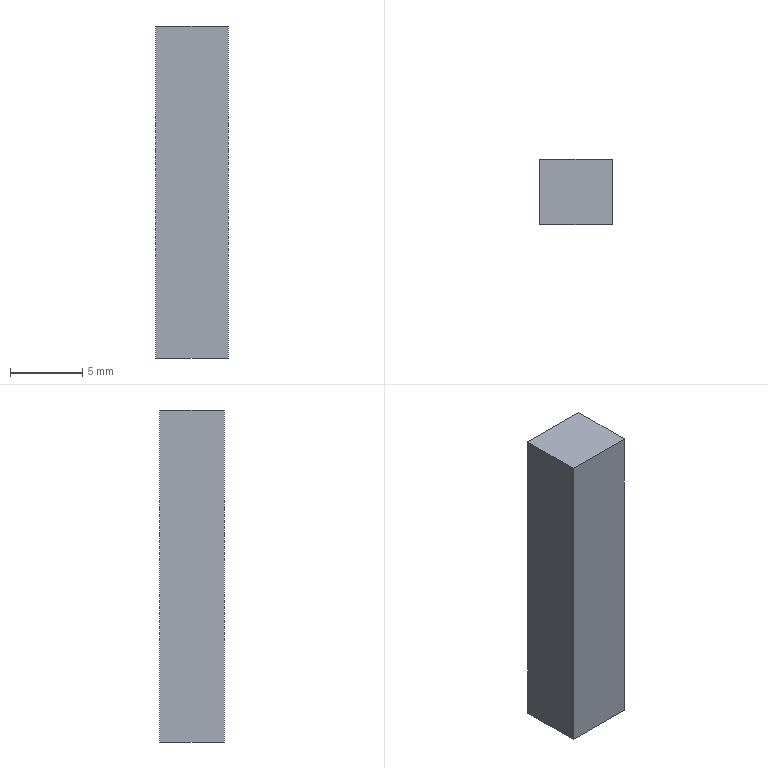Part | STEP file | Cuon T phu H01_71 | 1 solid | 6 faces | box 5 x 4.5 x 23 mm | volume 517.5 mm3 | plane 6
STEP:
#1=CARTESIAN_POINT('',(0.,0.,0.));
#2=DIRECTION('',(0.,0.,1.));
#3=DIRECTION('',(1.,0.,0.));
#4=AXIS2_PLACEMENT_3D('',#1,#2,#3);
#5=CARTESIAN_POINT('',(-2.5,2.25,-11.5));
#6=VERTEX_POINT('',#5);
#7=CARTESIAN_POINT('',(-2.5,-2.25,-11.5));
#8=VERTEX_POINT('',#7);
#9=CARTESIAN_POINT('',(-2.5,2.25,-11.5));
#10=DIRECTION('',(0.,-1.,0.));
#11=VECTOR('',#10,1.);
#12=LINE('',#9,#11);
#13=CARTESIAN_POINT('',(-2.5,2.25,11.5));
#14=DIRECTION('',(1.,0.,0.));
#15=DIRECTION('',(0.,1.,0.));
#16=AXIS2_PLACEMENT_3D('',#13,#14,#15);
#17=PLANE('',#16);
#18=CARTESIAN_POINT('',(0.,-23.));
#19=DIRECTION('',(-1.,0.));
#20=VECTOR('',#19,1.);
#21=LINE('',#18,#20);
#22=(GEOMETRIC_REPRESENTATION_CONTEXT(2)PARAMETRIC_REPRESENTATION_CONTEXT()REPRESENTATION_CONTEXT('',''));
#23=DEFINITIONAL_REPRESENTATION('',(#21),#22);
#24=PCURVE('',#17,#23);
#25=CARTESIAN_POINT('',(0.,0.,-11.5));
#26=DIRECTION('',(0.,0.,1.));
#27=DIRECTION('',(1.,0.,0.));
#28=AXIS2_PLACEMENT_3D('',#25,#26,#27);
#29=PLANE('',#28);
#30=CARTESIAN_POINT('',(-2.5,2.25));
#31=DIRECTION('',(0.,-1.));
#32=VECTOR('',#31,1.);
#33=LINE('',#30,#32);
#34=(GEOMETRIC_REPRESENTATION_CONTEXT(2)PARAMETRIC_REPRESENTATION_CONTEXT()REPRESENTATION_CONTEXT('',''));
#35=DEFINITIONAL_REPRESENTATION('',(#33),#34);
#36=PCURVE('',#29,#35);
#37=SURFACE_CURVE('',#12,(#24,#36),.PCURVE_S1.);
#38=EDGE_CURVE('',#6,#8,#37,.T.);
#39=ORIENTED_EDGE('',*,*,#38,.T.);
#40=CARTESIAN_POINT('',(-2.5,-2.25,11.5));
#41=VERTEX_POINT('',#40);
#42=CARTESIAN_POINT('',(-2.5,-2.25,11.5));
#43=DIRECTION('',(0.,0.,-1.));
#44=VECTOR('',#43,1.);
#45=LINE('',#42,#44);
#46=CARTESIAN_POINT('',(-4.5,0.));
#47=DIRECTION('',(0.,-1.));
#48=VECTOR('',#47,1.);
#49=LINE('',#46,#48);
#50=(GEOMETRIC_REPRESENTATION_CONTEXT(2)PARAMETRIC_REPRESENTATION_CONTEXT()REPRESENTATION_CONTEXT('',''));
#51=DEFINITIONAL_REPRESENTATION('',(#49),#50);
#52=PCURVE('',#17,#51);
#53=CARTESIAN_POINT('',(-2.5,-2.25,11.5));
#54=DIRECTION('',(0.,1.,0.));
#55=DIRECTION('',(0.,0.,1.));
#56=AXIS2_PLACEMENT_3D('',#53,#54,#55);
#57=PLANE('',#56);
#58=CARTESIAN_POINT('',(0.,0.));
#59=DIRECTION('',(-1.,0.));
#60=VECTOR('',#59,1.);
#61=LINE('',#58,#60);
#62=(GEOMETRIC_REPRESENTATION_CONTEXT(2)PARAMETRIC_REPRESENTATION_CONTEXT()REPRESENTATION_CONTEXT('',''));
#63=DEFINITIONAL_REPRESENTATION('',(#61),#62);
#64=PCURVE('',#57,#63);
#65=SURFACE_CURVE('',#45,(#52,#64),.PCURVE_S1.);
#66=EDGE_CURVE('',#41,#8,#65,.T.);
#67=ORIENTED_EDGE('',*,*,#66,.F.);
#68=CARTESIAN_POINT('',(-2.5,2.25,11.5));
#69=VERTEX_POINT('',#68);
#70=CARTESIAN_POINT('',(-2.5,2.25,11.5));
#71=DIRECTION('',(0.,-1.,0.));
#72=VECTOR('',#71,1.);
#73=LINE('',#70,#72);
#74=CARTESIAN_POINT('',(0.,0.));
#75=DIRECTION('',(-1.,0.));
#76=VECTOR('',#75,1.);
#77=LINE('',#74,#76);
#78=(GEOMETRIC_REPRESENTATION_CONTEXT(2)PARAMETRIC_REPRESENTATION_CONTEXT()REPRESENTATION_CONTEXT('',''));
#79=DEFINITIONAL_REPRESENTATION('',(#77),#78);
#80=PCURVE('',#17,#79);
#81=CARTESIAN_POINT('',(0.,0.,11.5));
#82=DIRECTION('',(0.,0.,1.));
#83=DIRECTION('',(1.,0.,0.));
#84=AXIS2_PLACEMENT_3D('',#81,#82,#83);
#85=PLANE('',#84);
#86=CARTESIAN_POINT('',(-2.5,2.25));
#87=DIRECTION('',(0.,-1.));
#88=VECTOR('',#87,1.);
#89=LINE('',#86,#88);
#90=(GEOMETRIC_REPRESENTATION_CONTEXT(2)PARAMETRIC_REPRESENTATION_CONTEXT()REPRESENTATION_CONTEXT('',''));
#91=DEFINITIONAL_REPRESENTATION('',(#89),#90);
#92=PCURVE('',#85,#91);
#93=SURFACE_CURVE('',#73,(#80,#92),.PCURVE_S1.);
#94=EDGE_CURVE('',#69,#41,#93,.T.);
#95=ORIENTED_EDGE('',*,*,#94,.F.);
#96=CARTESIAN_POINT('',(-2.5,2.25,11.5));
#97=DIRECTION('',(0.,0.,-1.));
#98=VECTOR('',#97,1.);
#99=LINE('',#96,#98);
#100=CARTESIAN_POINT('',(0.,0.));
#101=DIRECTION('',(0.,-1.));
#102=VECTOR('',#101,1.);
#103=LINE('',#100,#102);
#104=(GEOMETRIC_REPRESENTATION_CONTEXT(2)PARAMETRIC_REPRESENTATION_CONTEXT()REPRESENTATION_CONTEXT('',''));
#105=DEFINITIONAL_REPRESENTATION('',(#103),#104);
#106=PCURVE('',#17,#105);
#107=CARTESIAN_POINT('',(-2.5,2.25,11.5));
#108=DIRECTION('',(0.,-1.,0.));
#109=DIRECTION('',(0.,0.,-1.));
#110=AXIS2_PLACEMENT_3D('',#107,#108,#109);
#111=PLANE('',#110);
#112=CARTESIAN_POINT('',(0.,0.));
#113=DIRECTION('',(1.,0.));
#114=VECTOR('',#113,1.);
#115=LINE('',#112,#114);
#116=(GEOMETRIC_REPRESENTATION_CONTEXT(2)PARAMETRIC_REPRESENTATION_CONTEXT()REPRESENTATION_CONTEXT('',''));
#117=DEFINITIONAL_REPRESENTATION('',(#115),#116);
#118=PCURVE('',#111,#117);
#119=SURFACE_CURVE('',#99,(#106,#118),.PCURVE_S1.);
#120=EDGE_CURVE('',#69,#6,#119,.T.);
#121=ORIENTED_EDGE('',*,*,#120,.T.);
#122=EDGE_LOOP('',(#39,#67,#95,#121));
#123=FACE_BOUND('',#122,.T.);
#124=ADVANCED_FACE('',(#123),#17,.F.);
#125=CARTESIAN_POINT('',(2.5,-2.25,-11.5));
#126=VERTEX_POINT('',#125);
#127=CARTESIAN_POINT('',(-2.5,-2.25,-11.5));
#128=DIRECTION('',(1.,0.,0.));
#129=VECTOR('',#128,1.);
#130=LINE('',#127,#129);
#131=CARTESIAN_POINT('',(-23.,0.));
#132=DIRECTION('',(0.,1.));
#133=VECTOR('',#132,1.);
#134=LINE('',#131,#133);
#135=(GEOMETRIC_REPRESENTATION_CONTEXT(2)PARAMETRIC_REPRESENTATION_CONTEXT()REPRESENTATION_CONTEXT('',''));
#136=DEFINITIONAL_REPRESENTATION('',(#134),#135);
#137=PCURVE('',#57,#136);
#138=CARTESIAN_POINT('',(-2.5,-2.25));
#139=DIRECTION('',(1.,0.));
#140=VECTOR('',#139,1.);
#141=LINE('',#138,#140);
#142=(GEOMETRIC_REPRESENTATION_CONTEXT(2)PARAMETRIC_REPRESENTATION_CONTEXT()REPRESENTATION_CONTEXT('',''));
#143=DEFINITIONAL_REPRESENTATION('',(#141),#142);
#144=PCURVE('',#29,#143);
#145=SURFACE_CURVE('',#130,(#137,#144),.PCURVE_S1.);
#146=EDGE_CURVE('',#8,#126,#145,.T.);
#147=ORIENTED_EDGE('',*,*,#146,.T.);
#148=CARTESIAN_POINT('',(2.5,-2.25,11.5));
#149=VERTEX_POINT('',#148);
#150=CARTESIAN_POINT('',(2.5,-2.25,11.5));
#151=DIRECTION('',(0.,0.,-1.));
#152=VECTOR('',#151,1.);
#153=LINE('',#150,#152);
#154=CARTESIAN_POINT('',(0.,5.));
#155=DIRECTION('',(-1.,0.));
#156=VECTOR('',#155,1.);
#157=LINE('',#154,#156);
#158=(GEOMETRIC_REPRESENTATION_CONTEXT(2)PARAMETRIC_REPRESENTATION_CONTEXT()REPRESENTATION_CONTEXT('',''));
#159=DEFINITIONAL_REPRESENTATION('',(#157),#158);
#160=PCURVE('',#57,#159);
#161=CARTESIAN_POINT('',(2.5,2.25,11.5));
#162=DIRECTION('',(-1.,0.,0.));
#163=DIRECTION('',(0.,-1.,0.));
#164=AXIS2_PLACEMENT_3D('',#161,#162,#163);
#165=PLANE('',#164);
#166=CARTESIAN_POINT('',(4.5,0.));
#167=DIRECTION('',(0.,-1.));
#168=VECTOR('',#167,1.);
#169=LINE('',#166,#168);
#170=(GEOMETRIC_REPRESENTATION_CONTEXT(2)PARAMETRIC_REPRESENTATION_CONTEXT()REPRESENTATION_CONTEXT('',''));
#171=DEFINITIONAL_REPRESENTATION('',(#169),#170);
#172=PCURVE('',#165,#171);
#173=SURFACE_CURVE('',#153,(#160,#172),.PCURVE_S1.);
#174=EDGE_CURVE('',#149,#126,#173,.T.);
#175=ORIENTED_EDGE('',*,*,#174,.F.);
#176=CARTESIAN_POINT('',(-2.5,-2.25,11.5));
#177=DIRECTION('',(1.,0.,0.));
#178=VECTOR('',#177,1.);
#179=LINE('',#176,#178);
#180=CARTESIAN_POINT('',(0.,0.));
#181=DIRECTION('',(0.,1.));
#182=VECTOR('',#181,1.);
#183=LINE('',#180,#182);
#184=(GEOMETRIC_REPRESENTATION_CONTEXT(2)PARAMETRIC_REPRESENTATION_CONTEXT()REPRESENTATION_CONTEXT('',''));
#185=DEFINITIONAL_REPRESENTATION('',(#183),#184);
#186=PCURVE('',#57,#185);
#187=CARTESIAN_POINT('',(-2.5,-2.25));
#188=DIRECTION('',(1.,0.));
#189=VECTOR('',#188,1.);
#190=LINE('',#187,#189);
#191=(GEOMETRIC_REPRESENTATION_CONTEXT(2)PARAMETRIC_REPRESENTATION_CONTEXT()REPRESENTATION_CONTEXT('',''));
#192=DEFINITIONAL_REPRESENTATION('',(#190),#191);
#193=PCURVE('',#85,#192);
#194=SURFACE_CURVE('',#179,(#186,#193),.PCURVE_S1.);
#195=EDGE_CURVE('',#41,#149,#194,.T.);
#196=ORIENTED_EDGE('',*,*,#195,.F.);
#197=ORIENTED_EDGE('',*,*,#66,.T.);
#198=EDGE_LOOP('',(#147,#175,#196,#197));
#199=FACE_BOUND('',#198,.T.);
#200=ADVANCED_FACE('',(#199),#57,.F.);
#201=CARTESIAN_POINT('',(2.5,2.25,-11.5));
#202=VERTEX_POINT('',#201);
#203=CARTESIAN_POINT('',(2.5,2.25,-11.5));
#204=DIRECTION('',(0.,1.,0.));
#205=VECTOR('',#204,1.);
#206=LINE('',#203,#205);
#207=CARTESIAN_POINT('',(0.,-23.));
#208=DIRECTION('',(-1.,0.));
#209=VECTOR('',#208,1.);
#210=LINE('',#207,#209);
#211=(GEOMETRIC_REPRESENTATION_CONTEXT(2)PARAMETRIC_REPRESENTATION_CONTEXT()REPRESENTATION_CONTEXT('',''));
#212=DEFINITIONAL_REPRESENTATION('',(#210),#211);
#213=PCURVE('',#165,#212);
#214=CARTESIAN_POINT('',(2.5,2.25));
#215=DIRECTION('',(0.,1.));
#216=VECTOR('',#215,1.);
#217=LINE('',#214,#216);
#218=(GEOMETRIC_REPRESENTATION_CONTEXT(2)PARAMETRIC_REPRESENTATION_CONTEXT()REPRESENTATION_CONTEXT('',''));
#219=DEFINITIONAL_REPRESENTATION('',(#217),#218);
#220=PCURVE('',#29,#219);
#221=SURFACE_CURVE('',#206,(#213,#220),.PCURVE_S1.);
#222=EDGE_CURVE('',#126,#202,#221,.T.);
#223=ORIENTED_EDGE('',*,*,#222,.T.);
#224=CARTESIAN_POINT('',(2.5,2.25,11.5));
#225=VERTEX_POINT('',#224);
#226=CARTESIAN_POINT('',(2.5,2.25,11.5));
#227=DIRECTION('',(0.,0.,-1.));
#228=VECTOR('',#227,1.);
#229=LINE('',#226,#228);
#230=CARTESIAN_POINT('',(0.,0.));
#231=DIRECTION('',(0.,-1.));
#232=VECTOR('',#231,1.);
#233=LINE('',#230,#232);
#234=(GEOMETRIC_REPRESENTATION_CONTEXT(2)PARAMETRIC_REPRESENTATION_CONTEXT()REPRESENTATION_CONTEXT('',''));
#235=DEFINITIONAL_REPRESENTATION('',(#233),#234);
#236=PCURVE('',#165,#235);
#237=CARTESIAN_POINT('',(0.,5.));
#238=DIRECTION('',(1.,0.));
#239=VECTOR('',#238,1.);
#240=LINE('',#237,#239);
#241=(GEOMETRIC_REPRESENTATION_CONTEXT(2)PARAMETRIC_REPRESENTATION_CONTEXT()REPRESENTATION_CONTEXT('',''));
#242=DEFINITIONAL_REPRESENTATION('',(#240),#241);
#243=PCURVE('',#111,#242);
#244=SURFACE_CURVE('',#229,(#236,#243),.PCURVE_S1.);
#245=EDGE_CURVE('',#225,#202,#244,.T.);
#246=ORIENTED_EDGE('',*,*,#245,.F.);
#247=CARTESIAN_POINT('',(2.5,2.25,11.5));
#248=DIRECTION('',(0.,1.,0.));
#249=VECTOR('',#248,1.);
#250=LINE('',#247,#249);
#251=CARTESIAN_POINT('',(0.,0.));
#252=DIRECTION('',(-1.,0.));
#253=VECTOR('',#252,1.);
#254=LINE('',#251,#253);
#255=(GEOMETRIC_REPRESENTATION_CONTEXT(2)PARAMETRIC_REPRESENTATION_CONTEXT()REPRESENTATION_CONTEXT('',''));
#256=DEFINITIONAL_REPRESENTATION('',(#254),#255);
#257=PCURVE('',#165,#256);
#258=CARTESIAN_POINT('',(2.5,2.25));
#259=DIRECTION('',(0.,1.));
#260=VECTOR('',#259,1.);
#261=LINE('',#258,#260);
#262=(GEOMETRIC_REPRESENTATION_CONTEXT(2)PARAMETRIC_REPRESENTATION_CONTEXT()REPRESENTATION_CONTEXT('',''));
#263=DEFINITIONAL_REPRESENTATION('',(#261),#262);
#264=PCURVE('',#85,#263);
#265=SURFACE_CURVE('',#250,(#257,#264),.PCURVE_S1.);
#266=EDGE_CURVE('',#149,#225,#265,.T.);
#267=ORIENTED_EDGE('',*,*,#266,.F.);
#268=ORIENTED_EDGE('',*,*,#174,.T.);
#269=EDGE_LOOP('',(#223,#246,#267,#268));
#270=FACE_BOUND('',#269,.T.);
#271=ADVANCED_FACE('',(#270),#165,.F.);
#272=CARTESIAN_POINT('',(-2.5,2.25,-11.5));
#273=DIRECTION('',(-1.,0.,0.));
#274=VECTOR('',#273,1.);
#275=LINE('',#272,#274);
#276=CARTESIAN_POINT('',(23.,0.));
#277=DIRECTION('',(0.,-1.));
#278=VECTOR('',#277,1.);
#279=LINE('',#276,#278);
#280=(GEOMETRIC_REPRESENTATION_CONTEXT(2)PARAMETRIC_REPRESENTATION_CONTEXT()REPRESENTATION_CONTEXT('',''));
#281=DEFINITIONAL_REPRESENTATION('',(#279),#280);
#282=PCURVE('',#111,#281);
#283=CARTESIAN_POINT('',(-2.5,2.25));
#284=DIRECTION('',(-1.,0.));
#285=VECTOR('',#284,1.);
#286=LINE('',#283,#285);
#287=(GEOMETRIC_REPRESENTATION_CONTEXT(2)PARAMETRIC_REPRESENTATION_CONTEXT()REPRESENTATION_CONTEXT('',''));
#288=DEFINITIONAL_REPRESENTATION('',(#286),#287);
#289=PCURVE('',#29,#288);
#290=SURFACE_CURVE('',#275,(#282,#289),.PCURVE_S1.);
#291=EDGE_CURVE('',#202,#6,#290,.T.);
#292=ORIENTED_EDGE('',*,*,#291,.T.);
#293=ORIENTED_EDGE('',*,*,#120,.F.);
#294=CARTESIAN_POINT('',(-2.5,2.25,11.5));
#295=DIRECTION('',(-1.,0.,0.));
#296=VECTOR('',#295,1.);
#297=LINE('',#294,#296);
#298=CARTESIAN_POINT('',(0.,0.));
#299=DIRECTION('',(0.,-1.));
#300=VECTOR('',#299,1.);
#301=LINE('',#298,#300);
#302=(GEOMETRIC_REPRESENTATION_CONTEXT(2)PARAMETRIC_REPRESENTATION_CONTEXT()REPRESENTATION_CONTEXT('',''));
#303=DEFINITIONAL_REPRESENTATION('',(#301),#302);
#304=PCURVE('',#111,#303);
#305=CARTESIAN_POINT('',(-2.5,2.25));
#306=DIRECTION('',(-1.,0.));
#307=VECTOR('',#306,1.);
#308=LINE('',#305,#307);
#309=(GEOMETRIC_REPRESENTATION_CONTEXT(2)PARAMETRIC_REPRESENTATION_CONTEXT()REPRESENTATION_CONTEXT('',''));
#310=DEFINITIONAL_REPRESENTATION('',(#308),#309);
#311=PCURVE('',#85,#310);
#312=SURFACE_CURVE('',#297,(#304,#311),.PCURVE_S1.);
#313=EDGE_CURVE('',#225,#69,#312,.T.);
#314=ORIENTED_EDGE('',*,*,#313,.F.);
#315=ORIENTED_EDGE('',*,*,#245,.T.);
#316=EDGE_LOOP('',(#292,#293,#314,#315));
#317=FACE_BOUND('',#316,.T.);
#318=ADVANCED_FACE('',(#317),#111,.F.);
#319=ORIENTED_EDGE('',*,*,#94,.T.);
#320=ORIENTED_EDGE('',*,*,#195,.T.);
#321=ORIENTED_EDGE('',*,*,#266,.T.);
#322=ORIENTED_EDGE('',*,*,#313,.T.);
#323=EDGE_LOOP('',(#319,#320,#321,#322));
#324=FACE_BOUND('',#323,.T.);
#325=ADVANCED_FACE('',(#324),#85,.T.);
#326=ORIENTED_EDGE('',*,*,#38,.F.);
#327=ORIENTED_EDGE('',*,*,#291,.F.);
#328=ORIENTED_EDGE('',*,*,#222,.F.);
#329=ORIENTED_EDGE('',*,*,#146,.F.);
#330=EDGE_LOOP('',(#326,#327,#328,#329));
#331=FACE_BOUND('',#330,.T.);
#332=ADVANCED_FACE('',(#331),#29,.F.);
#333=CLOSED_SHELL('',(#124,#200,#271,#318,#325,#332));
#334=MANIFOLD_SOLID_BREP('',#333);
#335=(LENGTH_UNIT()NAMED_UNIT(*)SI_UNIT(.MILLI.,.METRE.));
#336=UNCERTAINTY_MEASURE_WITH_UNIT(LENGTH_MEASURE(0.0000001),#335,'','');
#337=(NAMED_UNIT(*)PLANE_ANGLE_UNIT()SI_UNIT($,.RADIAN.));
#338=(NAMED_UNIT(*)SI_UNIT($,.STERADIAN.)SOLID_ANGLE_UNIT());
#339=(GEOMETRIC_REPRESENTATION_CONTEXT(3)GLOBAL_UNCERTAINTY_ASSIGNED_CONTEXT((#336))GLOBAL_UNIT_ASSIGNED_CONTEXT((#335,#337,#338))REPRESENTATION_CONTEXT('',''));
#340=ADVANCED_BREP_SHAPE_REPRESENTATION('',(#4,#334),#339);